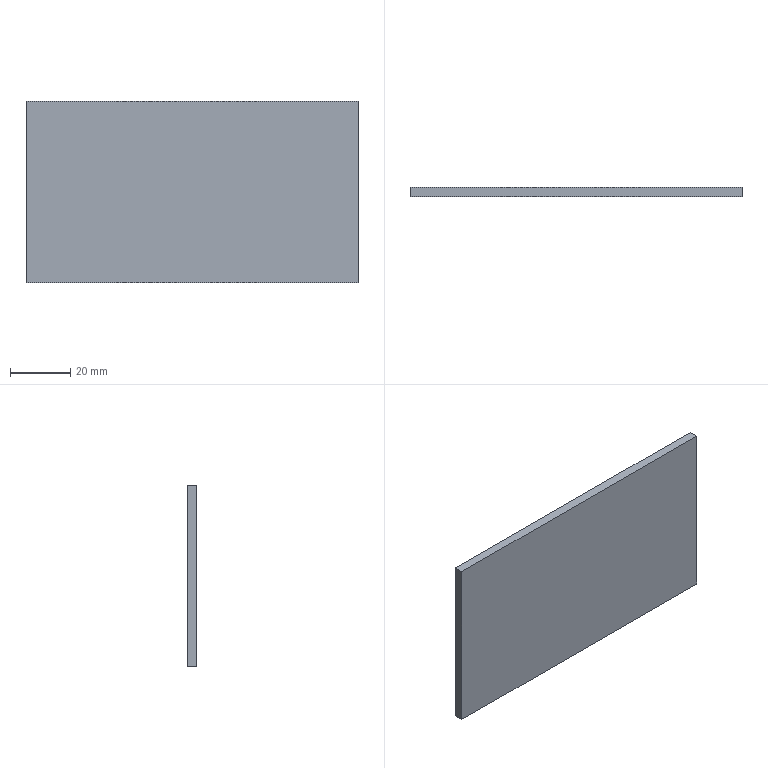Part | SolidWorks | features Extrusion 1 | 1 solid | 6 faces | box 110 x 3 x 60 mm | volume 19800 mm3 | plane 6
STEP:
#1=CARTESIAN_POINT('',(55.,0.,30.));
#2=VERTEX_POINT('',#1);
#3=CARTESIAN_POINT('',(55.,0.,-30.));
#4=VERTEX_POINT('',#3);
#5=CARTESIAN_POINT('',(55.,0.,30.));
#6=DIRECTION('',(0.,0.,-1.));
#7=VECTOR('',#6,1000.);
#8=LINE('',#5,#7);
#9=EDGE_CURVE('',#2,#4,#8,.T.);
#10=ORIENTED_EDGE('',*,*,#9,.T.);
#11=CARTESIAN_POINT('',(55.,3.,-30.));
#12=VERTEX_POINT('',#11);
#13=CARTESIAN_POINT('',(55.,3.,-30.));
#14=DIRECTION('',(0.,-1.,0.));
#15=VECTOR('',#14,1000.);
#16=LINE('',#13,#15);
#17=EDGE_CURVE('',#12,#4,#16,.T.);
#18=ORIENTED_EDGE('',*,*,#17,.F.);
#19=CARTESIAN_POINT('',(55.,3.,30.));
#20=VERTEX_POINT('',#19);
#21=CARTESIAN_POINT('',(55.,3.,30.));
#22=DIRECTION('',(0.,0.,-1.));
#23=VECTOR('',#22,1000.);
#24=LINE('',#21,#23);
#25=EDGE_CURVE('',#20,#12,#24,.T.);
#26=ORIENTED_EDGE('',*,*,#25,.F.);
#27=CARTESIAN_POINT('',(55.,3.,30.));
#28=DIRECTION('',(0.,-1.,0.));
#29=VECTOR('',#28,1000.);
#30=LINE('',#27,#29);
#31=EDGE_CURVE('',#20,#2,#30,.T.);
#32=ORIENTED_EDGE('',*,*,#31,.T.);
#33=EDGE_LOOP('',(#10,#18,#26,#32));
#34=FACE_OUTER_BOUND('',#33,.T.);
#35=CARTESIAN_POINT('',(55.,3.,30.));
#36=DIRECTION('',(-1.,0.,0.));
#37=DIRECTION('',(0.,0.,1.));
#38=AXIS2_PLACEMENT_3D('',#35,#36,#37);
#39=PLANE('',#38);
#40=ADVANCED_FACE('',(#34),#39,.F.);
#41=CARTESIAN_POINT('',(-55.,0.,-30.));
#42=VERTEX_POINT('',#41);
#43=CARTESIAN_POINT('',(-55.,0.,-30.));
#44=DIRECTION('',(-1.,0.,0.));
#45=VECTOR('',#44,1000.);
#46=LINE('',#43,#45);
#47=EDGE_CURVE('',#4,#42,#46,.T.);
#48=ORIENTED_EDGE('',*,*,#47,.T.);
#49=CARTESIAN_POINT('',(-55.,3.,-30.));
#50=VERTEX_POINT('',#49);
#51=CARTESIAN_POINT('',(-55.,3.,-30.));
#52=DIRECTION('',(0.,-1.,0.));
#53=VECTOR('',#52,1000.);
#54=LINE('',#51,#53);
#55=EDGE_CURVE('',#50,#42,#54,.T.);
#56=ORIENTED_EDGE('',*,*,#55,.F.);
#57=CARTESIAN_POINT('',(-55.,3.,-30.));
#58=DIRECTION('',(-1.,0.,0.));
#59=VECTOR('',#58,1000.);
#60=LINE('',#57,#59);
#61=EDGE_CURVE('',#12,#50,#60,.T.);
#62=ORIENTED_EDGE('',*,*,#61,.F.);
#63=ORIENTED_EDGE('',*,*,#17,.T.);
#64=EDGE_LOOP('',(#48,#56,#62,#63));
#65=FACE_OUTER_BOUND('',#64,.T.);
#66=CARTESIAN_POINT('',(-55.,3.,-30.));
#67=DIRECTION('',(0.,0.,1.));
#68=DIRECTION('',(1.,0.,0.));
#69=AXIS2_PLACEMENT_3D('',#66,#67,#68);
#70=PLANE('',#69);
#71=ADVANCED_FACE('',(#65),#70,.F.);
#72=CARTESIAN_POINT('',(-55.,0.,30.));
#73=VERTEX_POINT('',#72);
#74=CARTESIAN_POINT('',(-55.,0.,30.));
#75=DIRECTION('',(0.,0.,1.));
#76=VECTOR('',#75,1000.);
#77=LINE('',#74,#76);
#78=EDGE_CURVE('',#42,#73,#77,.T.);
#79=ORIENTED_EDGE('',*,*,#78,.T.);
#80=CARTESIAN_POINT('',(-55.,3.,30.));
#81=VERTEX_POINT('',#80);
#82=CARTESIAN_POINT('',(-55.,3.,30.));
#83=DIRECTION('',(0.,-1.,0.));
#84=VECTOR('',#83,1000.);
#85=LINE('',#82,#84);
#86=EDGE_CURVE('',#81,#73,#85,.T.);
#87=ORIENTED_EDGE('',*,*,#86,.F.);
#88=CARTESIAN_POINT('',(-55.,3.,30.));
#89=DIRECTION('',(0.,0.,1.));
#90=VECTOR('',#89,1000.);
#91=LINE('',#88,#90);
#92=EDGE_CURVE('',#50,#81,#91,.T.);
#93=ORIENTED_EDGE('',*,*,#92,.F.);
#94=ORIENTED_EDGE('',*,*,#55,.T.);
#95=EDGE_LOOP('',(#79,#87,#93,#94));
#96=FACE_OUTER_BOUND('',#95,.T.);
#97=CARTESIAN_POINT('',(-55.,3.,30.));
#98=DIRECTION('',(1.,0.,0.));
#99=DIRECTION('',(0.,0.,-1.));
#100=AXIS2_PLACEMENT_3D('',#97,#98,#99);
#101=PLANE('',#100);
#102=ADVANCED_FACE('',(#96),#101,.F.);
#103=CARTESIAN_POINT('',(-55.,0.,30.));
#104=DIRECTION('',(1.,0.,0.));
#105=VECTOR('',#104,1000.);
#106=LINE('',#103,#105);
#107=EDGE_CURVE('',#73,#2,#106,.T.);
#108=ORIENTED_EDGE('',*,*,#107,.T.);
#109=ORIENTED_EDGE('',*,*,#31,.F.);
#110=CARTESIAN_POINT('',(-55.,3.,30.));
#111=DIRECTION('',(1.,0.,0.));
#112=VECTOR('',#111,1000.);
#113=LINE('',#110,#112);
#114=EDGE_CURVE('',#81,#20,#113,.T.);
#115=ORIENTED_EDGE('',*,*,#114,.F.);
#116=ORIENTED_EDGE('',*,*,#86,.T.);
#117=EDGE_LOOP('',(#108,#109,#115,#116));
#118=FACE_OUTER_BOUND('',#117,.T.);
#119=CARTESIAN_POINT('',(-55.,3.,30.));
#120=DIRECTION('',(0.,0.,-1.));
#121=DIRECTION('',(-1.,0.,0.));
#122=AXIS2_PLACEMENT_3D('',#119,#120,#121);
#123=PLANE('',#122);
#124=ADVANCED_FACE('',(#118),#123,.F.);
#125=ORIENTED_EDGE('',*,*,#25,.T.);
#126=ORIENTED_EDGE('',*,*,#61,.T.);
#127=ORIENTED_EDGE('',*,*,#92,.T.);
#128=ORIENTED_EDGE('',*,*,#114,.T.);
#129=EDGE_LOOP('',(#125,#126,#127,#128));
#130=FACE_OUTER_BOUND('',#129,.T.);
#131=CARTESIAN_POINT('',(0.,3.,0.));
#132=DIRECTION('',(0.,-1.,0.));
#133=DIRECTION('',(0.,0.,-1.));
#134=AXIS2_PLACEMENT_3D('',#131,#132,#133);
#135=PLANE('',#134);
#136=ADVANCED_FACE('',(#130),#135,.F.);
#137=ORIENTED_EDGE('',*,*,#9,.F.);
#138=ORIENTED_EDGE('',*,*,#107,.F.);
#139=ORIENTED_EDGE('',*,*,#78,.F.);
#140=ORIENTED_EDGE('',*,*,#47,.F.);
#141=EDGE_LOOP('',(#137,#138,#139,#140));
#142=FACE_OUTER_BOUND('',#141,.T.);
#143=CARTESIAN_POINT('',(0.,0.,0.));
#144=DIRECTION('',(0.,-1.,0.));
#145=DIRECTION('',(0.,0.,-1.));
#146=AXIS2_PLACEMENT_3D('',#143,#144,#145);
#147=PLANE('',#146);
#148=ADVANCED_FACE('',(#142),#147,.T.);
#149=CLOSED_SHELL('',(#40,#71,#102,#124,#136,#148));
#150=MANIFOLD_SOLID_BREP('',#149);
#151=CARTESIAN_POINT('',(0.,0.,0.));
#152=DIRECTION('',(0.,0.,1.));
#153=DIRECTION('',(1.,0.,0.));
#154=AXIS2_PLACEMENT_3D('',#151,#152,#153);
#155=(LENGTH_UNIT()NAMED_UNIT(*)SI_UNIT(.MILLI.,.METRE.));
#156=UNCERTAINTY_MEASURE_WITH_UNIT(LENGTH_MEASURE(0.00001),#155,'','');
#157=(NAMED_UNIT(*)PLANE_ANGLE_UNIT()SI_UNIT($,.RADIAN.));
#158=(NAMED_UNIT(*)SI_UNIT($,.STERADIAN.)SOLID_ANGLE_UNIT());
#159=(GEOMETRIC_REPRESENTATION_CONTEXT(3)GLOBAL_UNCERTAINTY_ASSIGNED_CONTEXT((#156))GLOBAL_UNIT_ASSIGNED_CONTEXT((#155,#157,#158))REPRESENTATION_CONTEXT('',''));
#160=ADVANCED_BREP_SHAPE_REPRESENTATION('',(#150,#154),#159);